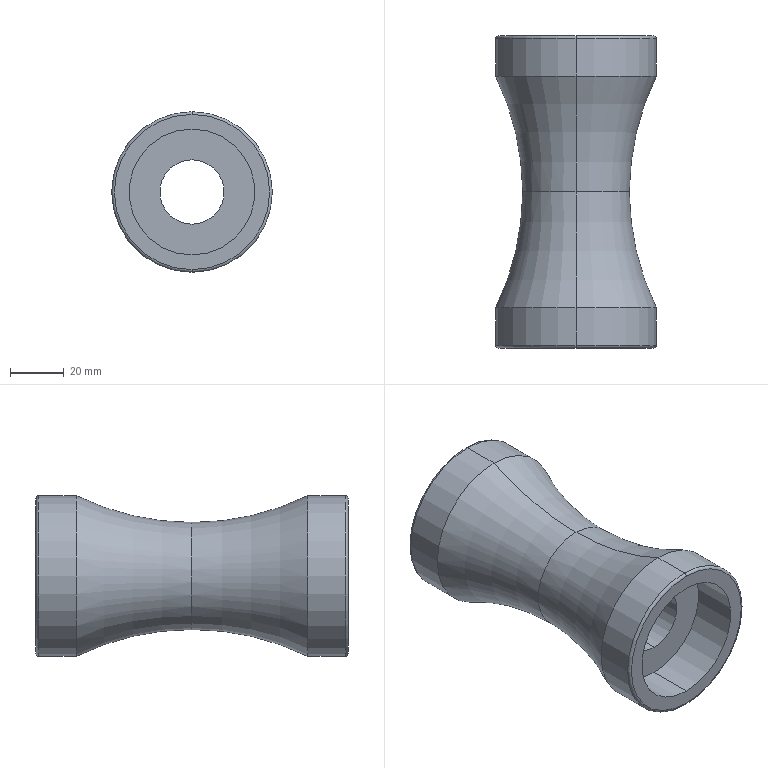Part | SolidWorks | features ICE 3, Fillet 1, Revolution 1 | 1 solid | 22 faces | box 60 x 116.5 x 60 mm | volume 137866 mm3 | cylinder 10 | torus 8 | plane 4 | commonest cylinder face diameters 47 x4 60 x4 24 x2
STEP:
#1=CARTESIAN_POINT('',(0.,15.,-30.));
#2=VERTEX_POINT('',#1);
#3=CARTESIAN_POINT('',(0.,58.25,-20.));
#4=VERTEX_POINT('',#3);
#5=CARTESIAN_POINT('',(0.,58.25,-118.528));
#6=DIRECTION('',(-1.,0.,0.));
#7=DIRECTION('',(0.,0.,1.));
#8=AXIS2_PLACEMENT_3D('',#5,#6,#7);
#9=CIRCLE('',#8,98.528);
#10=EDGE_CURVE('',#2,#4,#9,.T.);
#11=ORIENTED_EDGE('',*,*,#10,.T.);
#12=CARTESIAN_POINT('',(0.,58.25,20.));
#13=VERTEX_POINT('',#12);
#14=CARTESIAN_POINT('',(0.,58.25,0.));
#15=DIRECTION('',(0.,-1.,0.));
#16=DIRECTION('',(0.,0.,-1.));
#17=AXIS2_PLACEMENT_3D('',#14,#15,#16);
#18=CIRCLE('',#17,20.);
#19=EDGE_CURVE('',#4,#13,#18,.T.);
#20=ORIENTED_EDGE('',*,*,#19,.T.);
#21=CARTESIAN_POINT('',(0.,15.,30.));
#22=VERTEX_POINT('',#21);
#23=CARTESIAN_POINT('',(0.,58.25,118.528));
#24=DIRECTION('',(1.,0.,0.));
#25=DIRECTION('',(0.,0.,-1.));
#26=AXIS2_PLACEMENT_3D('',#23,#24,#25);
#27=CIRCLE('',#26,98.528);
#28=EDGE_CURVE('',#22,#13,#27,.T.);
#29=ORIENTED_EDGE('',*,*,#28,.F.);
#30=CARTESIAN_POINT('',(0.,15.,0.));
#31=DIRECTION('',(0.,-1.,0.));
#32=DIRECTION('',(0.,0.,-1.));
#33=AXIS2_PLACEMENT_3D('',#30,#31,#32);
#34=CIRCLE('',#33,30.);
#35=EDGE_CURVE('',#2,#22,#34,.T.);
#36=ORIENTED_EDGE('',*,*,#35,.F.);
#37=EDGE_LOOP('',(#11,#20,#29,#36));
#38=FACE_OUTER_BOUND('',#37,.T.);
#39=CARTESIAN_POINT('',(0.,58.25,0.));
#40=DIRECTION('',(0.,-1.,0.));
#41=DIRECTION('',(0.,0.,-1.));
#42=AXIS2_PLACEMENT_3D('',#39,#40,#41);
#43=TOROIDAL_SURFACE('',#42,118.528,98.528);
#44=ADVANCED_FACE('',(#38),#43,.F.);
#45=ORIENTED_EDGE('',*,*,#28,.T.);
#46=CARTESIAN_POINT('',(0.,58.25,0.));
#47=DIRECTION('',(0.,-1.,0.));
#48=DIRECTION('',(0.,0.,-1.));
#49=AXIS2_PLACEMENT_3D('',#46,#47,#48);
#50=CIRCLE('',#49,20.);
#51=EDGE_CURVE('',#13,#4,#50,.T.);
#52=ORIENTED_EDGE('',*,*,#51,.T.);
#53=ORIENTED_EDGE('',*,*,#10,.F.);
#54=CARTESIAN_POINT('',(0.,15.,0.));
#55=DIRECTION('',(0.,-1.,0.));
#56=DIRECTION('',(0.,0.,-1.));
#57=AXIS2_PLACEMENT_3D('',#54,#55,#56);
#58=CIRCLE('',#57,30.);
#59=EDGE_CURVE('',#22,#2,#58,.T.);
#60=ORIENTED_EDGE('',*,*,#59,.F.);
#61=EDGE_LOOP('',(#45,#52,#53,#60));
#62=FACE_OUTER_BOUND('',#61,.T.);
#63=CARTESIAN_POINT('',(0.,58.25,0.));
#64=DIRECTION('',(0.,-1.,0.));
#65=DIRECTION('',(0.,0.,-1.));
#66=AXIS2_PLACEMENT_3D('',#63,#64,#65);
#67=TOROIDAL_SURFACE('',#66,118.528,98.528);
#68=ADVANCED_FACE('',(#62),#67,.F.);
#69=CARTESIAN_POINT('',(0.,1.,30.));
#70=VERTEX_POINT('',#69);
#71=CARTESIAN_POINT('',(0.,1.,-30.));
#72=VERTEX_POINT('',#71);
#73=CARTESIAN_POINT('',(0.,1.,0.));
#74=DIRECTION('',(0.,1.,0.));
#75=DIRECTION('',(0.,0.,-1.));
#76=AXIS2_PLACEMENT_3D('',#73,#74,#75);
#77=CIRCLE('',#76,30.);
#78=EDGE_CURVE('',#70,#72,#77,.T.);
#79=ORIENTED_EDGE('',*,*,#78,.F.);
#80=CARTESIAN_POINT('',(0.,0.,29.));
#81=VERTEX_POINT('',#80);
#82=CARTESIAN_POINT('',(0.,1.,29.));
#83=DIRECTION('',(1.,0.,0.));
#84=DIRECTION('',(0.,0.,-1.));
#85=AXIS2_PLACEMENT_3D('',#82,#83,#84);
#86=CIRCLE('',#85,1.);
#87=EDGE_CURVE('',#70,#81,#86,.T.);
#88=ORIENTED_EDGE('',*,*,#87,.T.);
#89=CARTESIAN_POINT('',(0.,0.,-29.));
#90=VERTEX_POINT('',#89);
#91=CARTESIAN_POINT('',(0.,0.,0.));
#92=DIRECTION('',(0.,-1.,0.));
#93=DIRECTION('',(0.,0.,-1.));
#94=AXIS2_PLACEMENT_3D('',#91,#92,#93);
#95=CIRCLE('',#94,29.);
#96=EDGE_CURVE('',#90,#81,#95,.T.);
#97=ORIENTED_EDGE('',*,*,#96,.F.);
#98=CARTESIAN_POINT('',(0.,1.,-29.));
#99=DIRECTION('',(-1.,0.,0.));
#100=DIRECTION('',(0.,0.,1.));
#101=AXIS2_PLACEMENT_3D('',#98,#99,#100);
#102=CIRCLE('',#101,1.);
#103=EDGE_CURVE('',#72,#90,#102,.T.);
#104=ORIENTED_EDGE('',*,*,#103,.F.);
#105=EDGE_LOOP('',(#79,#88,#97,#104));
#106=FACE_OUTER_BOUND('',#105,.T.);
#107=CARTESIAN_POINT('',(0.,1.,0.));
#108=DIRECTION('',(0.,-1.,0.));
#109=DIRECTION('',(0.,0.,-1.));
#110=AXIS2_PLACEMENT_3D('',#107,#108,#109);
#111=TOROIDAL_SURFACE('',#110,29.,1.);
#112=ADVANCED_FACE('',(#106),#111,.T.);
#113=CARTESIAN_POINT('',(0.,115.5,-30.));
#114=VERTEX_POINT('',#113);
#115=CARTESIAN_POINT('',(0.,115.5,30.));
#116=VERTEX_POINT('',#115);
#117=CARTESIAN_POINT('',(0.,115.5,0.));
#118=DIRECTION('',(0.,-1.,0.));
#119=DIRECTION('',(0.,0.,1.));
#120=AXIS2_PLACEMENT_3D('',#117,#118,#119);
#121=CIRCLE('',#120,30.);
#122=EDGE_CURVE('',#114,#116,#121,.T.);
#123=ORIENTED_EDGE('',*,*,#122,.F.);
#124=CARTESIAN_POINT('',(0.,116.5,-29.));
#125=VERTEX_POINT('',#124);
#126=CARTESIAN_POINT('',(0.,115.5,-29.));
#127=DIRECTION('',(1.,0.,0.));
#128=DIRECTION('',(0.,0.,-1.));
#129=AXIS2_PLACEMENT_3D('',#126,#127,#128);
#130=CIRCLE('',#129,1.);
#131=EDGE_CURVE('',#114,#125,#130,.T.);
#132=ORIENTED_EDGE('',*,*,#131,.T.);
#133=CARTESIAN_POINT('',(0.,116.5,29.));
#134=VERTEX_POINT('',#133);
#135=CARTESIAN_POINT('',(0.,116.5,0.));
#136=DIRECTION('',(0.,1.,0.));
#137=DIRECTION('',(0.,0.,1.));
#138=AXIS2_PLACEMENT_3D('',#135,#136,#137);
#139=CIRCLE('',#138,29.);
#140=EDGE_CURVE('',#134,#125,#139,.T.);
#141=ORIENTED_EDGE('',*,*,#140,.F.);
#142=CARTESIAN_POINT('',(0.,115.5,29.));
#143=DIRECTION('',(-1.,0.,0.));
#144=DIRECTION('',(0.,0.,1.));
#145=AXIS2_PLACEMENT_3D('',#142,#143,#144);
#146=CIRCLE('',#145,1.);
#147=EDGE_CURVE('',#116,#134,#146,.T.);
#148=ORIENTED_EDGE('',*,*,#147,.F.);
#149=EDGE_LOOP('',(#123,#132,#141,#148));
#150=FACE_OUTER_BOUND('',#149,.T.);
#151=CARTESIAN_POINT('',(0.,115.5,0.));
#152=DIRECTION('',(0.,1.,0.));
#153=DIRECTION('',(0.,0.,1.));
#154=AXIS2_PLACEMENT_3D('',#151,#152,#153);
#155=TOROIDAL_SURFACE('',#154,29.,1.);
#156=ADVANCED_FACE('',(#150),#155,.T.);
#157=CARTESIAN_POINT('',(0.,17.,23.5));
#158=VERTEX_POINT('',#157);
#159=CARTESIAN_POINT('',(0.,17.,-23.5));
#160=VERTEX_POINT('',#159);
#161=CARTESIAN_POINT('',(0.,17.,0.));
#162=DIRECTION('',(0.,-1.,0.));
#163=DIRECTION('',(0.,0.,-1.));
#164=AXIS2_PLACEMENT_3D('',#161,#162,#163);
#165=CIRCLE('',#164,23.5);
#166=EDGE_CURVE('',#158,#160,#165,.T.);
#167=ORIENTED_EDGE('',*,*,#166,.F.);
#168=CARTESIAN_POINT('',(0.,0.,23.5));
#169=VERTEX_POINT('',#168);
#170=CARTESIAN_POINT('',(0.,17.,23.5));
#171=DIRECTION('',(0.,-1.,0.));
#172=VECTOR('',#171,1000.);
#173=LINE('',#170,#172);
#174=EDGE_CURVE('',#158,#169,#173,.T.);
#175=ORIENTED_EDGE('',*,*,#174,.T.);
#176=CARTESIAN_POINT('',(0.,0.,-23.5));
#177=VERTEX_POINT('',#176);
#178=CARTESIAN_POINT('',(0.,0.,0.));
#179=DIRECTION('',(0.,-1.,0.));
#180=DIRECTION('',(0.,0.,-1.));
#181=AXIS2_PLACEMENT_3D('',#178,#179,#180);
#182=CIRCLE('',#181,23.5);
#183=EDGE_CURVE('',#169,#177,#182,.T.);
#184=ORIENTED_EDGE('',*,*,#183,.T.);
#185=CARTESIAN_POINT('',(0.,17.,-23.5));
#186=DIRECTION('',(0.,-1.,0.));
#187=VECTOR('',#186,1000.);
#188=LINE('',#185,#187);
#189=EDGE_CURVE('',#160,#177,#188,.T.);
#190=ORIENTED_EDGE('',*,*,#189,.F.);
#191=EDGE_LOOP('',(#167,#175,#184,#190));
#192=FACE_OUTER_BOUND('',#191,.T.);
#193=CARTESIAN_POINT('',(0.,17.,0.));
#194=DIRECTION('',(0.,-1.,0.));
#195=DIRECTION('',(0.,0.,-1.));
#196=AXIS2_PLACEMENT_3D('',#193,#194,#195);
#197=CYLINDRICAL_SURFACE('',#196,23.5);
#198=ADVANCED_FACE('',(#192),#197,.F.);
#199=CARTESIAN_POINT('',(0.,99.5,-23.5));
#200=VERTEX_POINT('',#199);
#201=CARTESIAN_POINT('',(0.,99.5,23.5));
#202=VERTEX_POINT('',#201);
#203=CARTESIAN_POINT('',(0.,99.5,0.));
#204=DIRECTION('',(0.,1.,0.));
#205=DIRECTION('',(0.,0.,1.));
#206=AXIS2_PLACEMENT_3D('',#203,#204,#205);
#207=CIRCLE('',#206,23.5);
#208=EDGE_CURVE('',#200,#202,#207,.T.);
#209=ORIENTED_EDGE('',*,*,#208,.F.);
#210=CARTESIAN_POINT('',(0.,116.5,-23.5));
#211=VERTEX_POINT('',#210);
#212=CARTESIAN_POINT('',(0.,99.5,-23.5));
#213=DIRECTION('',(0.,1.,0.));
#214=VECTOR('',#213,1000.);
#215=LINE('',#212,#214);
#216=EDGE_CURVE('',#200,#211,#215,.T.);
#217=ORIENTED_EDGE('',*,*,#216,.T.);
#218=CARTESIAN_POINT('',(0.,116.5,23.5));
#219=VERTEX_POINT('',#218);
#220=CARTESIAN_POINT('',(0.,116.5,0.));
#221=DIRECTION('',(0.,1.,0.));
#222=DIRECTION('',(0.,0.,1.));
#223=AXIS2_PLACEMENT_3D('',#220,#221,#222);
#224=CIRCLE('',#223,23.5);
#225=EDGE_CURVE('',#211,#219,#224,.T.);
#226=ORIENTED_EDGE('',*,*,#225,.T.);
#227=CARTESIAN_POINT('',(0.,99.5,23.5));
#228=DIRECTION('',(0.,1.,0.));
#229=VECTOR('',#228,1000.);
#230=LINE('',#227,#229);
#231=EDGE_CURVE('',#202,#219,#230,.T.);
#232=ORIENTED_EDGE('',*,*,#231,.F.);
#233=EDGE_LOOP('',(#209,#217,#226,#232));
#234=FACE_OUTER_BOUND('',#233,.T.);
#235=CARTESIAN_POINT('',(0.,99.5,0.));
#236=DIRECTION('',(0.,1.,0.));
#237=DIRECTION('',(0.,0.,1.));
#238=AXIS2_PLACEMENT_3D('',#235,#236,#237);
#239=CYLINDRICAL_SURFACE('',#238,23.5);
#240=ADVANCED_FACE('',(#234),#239,.F.);
#241=ORIENTED_EDGE('',*,*,#122,.T.);
#242=CARTESIAN_POINT('',(0.,101.5,30.));
#243=VERTEX_POINT('',#242);
#244=CARTESIAN_POINT('',(0.,0.,30.));
#245=DIRECTION('',(0.,-1.,0.));
#246=VECTOR('',#245,1000.);
#247=LINE('',#244,#246);
#248=EDGE_CURVE('',#116,#243,#247,.T.);
#249=ORIENTED_EDGE('',*,*,#248,.T.);
#250=CARTESIAN_POINT('',(0.,101.5,-30.));
#251=VERTEX_POINT('',#250);
#252=CARTESIAN_POINT('',(0.,101.5,0.));
#253=DIRECTION('',(0.,-1.,0.));
#254=DIRECTION('',(0.,0.,-1.));
#255=AXIS2_PLACEMENT_3D('',#252,#253,#254);
#256=CIRCLE('',#255,30.);
#257=EDGE_CURVE('',#251,#243,#256,.T.);
#258=ORIENTED_EDGE('',*,*,#257,.F.);
#259=CARTESIAN_POINT('',(0.,0.,-30.));
#260=DIRECTION('',(0.,-1.,0.));
#261=VECTOR('',#260,1000.);
#262=LINE('',#259,#261);
#263=EDGE_CURVE('',#114,#251,#262,.T.);
#264=ORIENTED_EDGE('',*,*,#263,.F.);
#265=EDGE_LOOP('',(#241,#249,#258,#264));
#266=FACE_OUTER_BOUND('',#265,.T.);
#267=CARTESIAN_POINT('',(0.,0.,0.));
#268=DIRECTION('',(0.,-1.,0.));
#269=DIRECTION('',(0.,0.,-1.));
#270=AXIS2_PLACEMENT_3D('',#267,#268,#269);
#271=CYLINDRICAL_SURFACE('',#270,30.);
#272=ADVANCED_FACE('',(#266),#271,.T.);
#273=ORIENTED_EDGE('',*,*,#51,.F.);
#274=CARTESIAN_POINT('',(0.,58.25,118.528));
#275=DIRECTION('',(1.,0.,0.));
#276=DIRECTION('',(0.,0.,-1.));
#277=AXIS2_PLACEMENT_3D('',#274,#275,#276);
#278=CIRCLE('',#277,98.528);
#279=EDGE_CURVE('',#13,#243,#278,.T.);
#280=ORIENTED_EDGE('',*,*,#279,.T.);
#281=CARTESIAN_POINT('',(0.,101.5,0.));
#282=DIRECTION('',(0.,-1.,0.));
#283=DIRECTION('',(0.,0.,-1.));
#284=AXIS2_PLACEMENT_3D('',#281,#282,#283);
#285=CIRCLE('',#284,30.);
#286=EDGE_CURVE('',#243,#251,#285,.T.);
#287=ORIENTED_EDGE('',*,*,#286,.T.);
#288=CARTESIAN_POINT('',(0.,58.25,-118.528));
#289=DIRECTION('',(-1.,0.,0.));
#290=DIRECTION('',(0.,0.,1.));
#291=AXIS2_PLACEMENT_3D('',#288,#289,#290);
#292=CIRCLE('',#291,98.528);
#293=EDGE_CURVE('',#4,#251,#292,.T.);
#294=ORIENTED_EDGE('',*,*,#293,.F.);
#295=EDGE_LOOP('',(#273,#280,#287,#294));
#296=FACE_OUTER_BOUND('',#295,.T.);
#297=CARTESIAN_POINT('',(0.,58.25,0.));
#298=DIRECTION('',(0.,-1.,0.));
#299=DIRECTION('',(0.,0.,-1.));
#300=AXIS2_PLACEMENT_3D('',#297,#298,#299);
#301=TOROIDAL_SURFACE('',#300,118.528,98.528);
#302=ADVANCED_FACE('',(#296),#301,.F.);
#303=ORIENTED_EDGE('',*,*,#35,.T.);
#304=CARTESIAN_POINT('',(0.,0.,30.));
#305=DIRECTION('',(0.,-1.,0.));
#306=VECTOR('',#305,1000.);
#307=LINE('',#304,#306);
#308=EDGE_CURVE('',#22,#70,#307,.T.);
#309=ORIENTED_EDGE('',*,*,#308,.T.);
#310=ORIENTED_EDGE('',*,*,#78,.T.);
#311=CARTESIAN_POINT('',(0.,0.,-30.));
#312=DIRECTION('',(0.,-1.,0.));
#313=VECTOR('',#312,1000.);
#314=LINE('',#311,#313);
#315=EDGE_CURVE('',#2,#72,#314,.T.);
#316=ORIENTED_EDGE('',*,*,#315,.F.);
#317=EDGE_LOOP('',(#303,#309,#310,#316));
#318=FACE_OUTER_BOUND('',#317,.T.);
#319=CARTESIAN_POINT('',(0.,0.,0.));
#320=DIRECTION('',(0.,-1.,0.));
#321=DIRECTION('',(0.,0.,-1.));
#322=AXIS2_PLACEMENT_3D('',#319,#320,#321);
#323=CYLINDRICAL_SURFACE('',#322,30.);
#324=ADVANCED_FACE('',(#318),#323,.T.);
#325=CARTESIAN_POINT('',(0.,17.,-12.));
#326=VERTEX_POINT('',#325);
#327=CARTESIAN_POINT('',(0.,17.,12.));
#328=VERTEX_POINT('',#327);
#329=CARTESIAN_POINT('',(0.,17.,0.));
#330=DIRECTION('',(0.,1.,0.));
#331=DIRECTION('',(0.,0.,-1.));
#332=AXIS2_PLACEMENT_3D('',#329,#330,#331);
#333=CIRCLE('',#332,12.);
#334=EDGE_CURVE('',#326,#328,#333,.T.);
#335=ORIENTED_EDGE('',*,*,#334,.F.);
#336=CARTESIAN_POINT('',(0.,99.5,-12.));
#337=VERTEX_POINT('',#336);
#338=CARTESIAN_POINT('',(0.,-33.941,-12.));
#339=DIRECTION('',(0.,1.,0.));
#340=VECTOR('',#339,1000.);
#341=LINE('',#338,#340);
#342=EDGE_CURVE('',#326,#337,#341,.T.);
#343=ORIENTED_EDGE('',*,*,#342,.T.);
#344=CARTESIAN_POINT('',(0.,99.5,12.));
#345=VERTEX_POINT('',#344);
#346=CARTESIAN_POINT('',(0.,99.5,0.));
#347=DIRECTION('',(0.,-1.,0.));
#348=DIRECTION('',(0.,0.,1.));
#349=AXIS2_PLACEMENT_3D('',#346,#347,#348);
#350=CIRCLE('',#349,12.);
#351=EDGE_CURVE('',#345,#337,#350,.T.);
#352=ORIENTED_EDGE('',*,*,#351,.F.);
#353=CARTESIAN_POINT('',(0.,-33.941,12.));
#354=DIRECTION('',(0.,1.,0.));
#355=VECTOR('',#354,1000.);
#356=LINE('',#353,#355);
#357=EDGE_CURVE('',#328,#345,#356,.T.);
#358=ORIENTED_EDGE('',*,*,#357,.F.);
#359=EDGE_LOOP('',(#335,#343,#352,#358));
#360=FACE_OUTER_BOUND('',#359,.T.);
#361=CARTESIAN_POINT('',(0.,-33.941,0.));
#362=DIRECTION('',(0.,1.,0.));
#363=DIRECTION('',(0.,0.,1.));
#364=AXIS2_PLACEMENT_3D('',#361,#362,#363);
#365=CYLINDRICAL_SURFACE('',#364,12.);
#366=ADVANCED_FACE('',(#360),#365,.F.);
#367=ORIENTED_EDGE('',*,*,#342,.F.);
#368=CARTESIAN_POINT('',(0.,17.,0.));
#369=DIRECTION('',(0.,1.,0.));
#370=DIRECTION('',(0.,0.,-1.));
#371=AXIS2_PLACEMENT_3D('',#368,#369,#370);
#372=CIRCLE('',#371,12.);
#373=EDGE_CURVE('',#328,#326,#372,.T.);
#374=ORIENTED_EDGE('',*,*,#373,.F.);
#375=ORIENTED_EDGE('',*,*,#357,.T.);
#376=CARTESIAN_POINT('',(0.,99.5,0.));
#377=DIRECTION('',(0.,-1.,0.));
#378=DIRECTION('',(0.,0.,1.));
#379=AXIS2_PLACEMENT_3D('',#376,#377,#378);
#380=CIRCLE('',#379,12.);
#381=EDGE_CURVE('',#337,#345,#380,.T.);
#382=ORIENTED_EDGE('',*,*,#381,.F.);
#383=EDGE_LOOP('',(#367,#374,#375,#382));
#384=FACE_OUTER_BOUND('',#383,.T.);
#385=CARTESIAN_POINT('',(0.,-33.941,0.));
#386=DIRECTION('',(0.,1.,0.));
#387=DIRECTION('',(0.,0.,1.));
#388=AXIS2_PLACEMENT_3D('',#385,#386,#387);
#389=CYLINDRICAL_SURFACE('',#388,12.);
#390=ADVANCED_FACE('',(#384),#389,.F.);
#391=ORIENTED_EDGE('',*,*,#96,.T.);
#392=CARTESIAN_POINT('',(0.,0.,0.));
#393=DIRECTION('',(0.,-1.,0.));
#394=DIRECTION('',(0.,0.,-1.));
#395=AXIS2_PLACEMENT_3D('',#392,#393,#394);
#396=CIRCLE('',#395,29.);
#397=EDGE_CURVE('',#81,#90,#396,.T.);
#398=ORIENTED_EDGE('',*,*,#397,.T.);
#399=EDGE_LOOP('',(#391,#398));
#400=FACE_OUTER_BOUND('',#399,.T.);
#401=CARTESIAN_POINT('',(0.,0.,0.));
#402=DIRECTION('',(0.,-1.,0.));
#403=DIRECTION('',(0.,0.,-1.));
#404=AXIS2_PLACEMENT_3D('',#401,#402,#403);
#405=CIRCLE('',#404,23.5);
#406=EDGE_CURVE('',#177,#169,#405,.T.);
#407=ORIENTED_EDGE('',*,*,#406,.F.);
#408=ORIENTED_EDGE('',*,*,#183,.F.);
#409=EDGE_LOOP('',(#407,#408));
#410=FACE_BOUND('',#409,.T.);
#411=CARTESIAN_POINT('',(0.,0.,0.));
#412=DIRECTION('',(0.,-1.,0.));
#413=DIRECTION('',(0.,0.,-1.));
#414=AXIS2_PLACEMENT_3D('',#411,#412,#413);
#415=PLANE('',#414);
#416=ADVANCED_FACE('',(#400,#410),#415,.T.);
#417=ORIENTED_EDGE('',*,*,#308,.F.);
#418=ORIENTED_EDGE('',*,*,#59,.T.);
#419=ORIENTED_EDGE('',*,*,#315,.T.);
#420=CARTESIAN_POINT('',(0.,1.,0.));
#421=DIRECTION('',(0.,1.,0.));
#422=DIRECTION('',(0.,0.,-1.));
#423=AXIS2_PLACEMENT_3D('',#420,#421,#422);
#424=CIRCLE('',#423,30.);
#425=EDGE_CURVE('',#72,#70,#424,.T.);
#426=ORIENTED_EDGE('',*,*,#425,.T.);
#427=EDGE_LOOP('',(#417,#418,#419,#426));
#428=FACE_OUTER_BOUND('',#427,.T.);
#429=CARTESIAN_POINT('',(0.,0.,0.));
#430=DIRECTION('',(0.,-1.,0.));
#431=DIRECTION('',(0.,0.,-1.));
#432=AXIS2_PLACEMENT_3D('',#429,#430,#431);
#433=CYLINDRICAL_SURFACE('',#432,30.);
#434=ADVANCED_FACE('',(#428),#433,.T.);
#435=ORIENTED_EDGE('',*,*,#19,.F.);
#436=ORIENTED_EDGE('',*,*,#293,.T.);
#437=ORIENTED_EDGE('',*,*,#257,.T.);
#438=ORIENTED_EDGE('',*,*,#279,.F.);
#439=EDGE_LOOP('',(#435,#436,#437,#438));
#440=FACE_OUTER_BOUND('',#439,.T.);
#441=CARTESIAN_POINT('',(0.,58.25,0.));
#442=DIRECTION('',(0.,-1.,0.));
#443=DIRECTION('',(0.,0.,-1.));
#444=AXIS2_PLACEMENT_3D('',#441,#442,#443);
#445=TOROIDAL_SURFACE('',#444,118.528,98.528);
#446=ADVANCED_FACE('',(#440),#445,.F.);
#447=ORIENTED_EDGE('',*,*,#248,.F.);
#448=CARTESIAN_POINT('',(0.,115.5,0.));
#449=DIRECTION('',(0.,-1.,0.));
#450=DIRECTION('',(0.,0.,1.));
#451=AXIS2_PLACEMENT_3D('',#448,#449,#450);
#452=CIRCLE('',#451,30.);
#453=EDGE_CURVE('',#116,#114,#452,.T.);
#454=ORIENTED_EDGE('',*,*,#453,.T.);
#455=ORIENTED_EDGE('',*,*,#263,.T.);
#456=ORIENTED_EDGE('',*,*,#286,.F.);
#457=EDGE_LOOP('',(#447,#454,#455,#456));
#458=FACE_OUTER_BOUND('',#457,.T.);
#459=CARTESIAN_POINT('',(0.,0.,0.));
#460=DIRECTION('',(0.,-1.,0.));
#461=DIRECTION('',(0.,0.,-1.));
#462=AXIS2_PLACEMENT_3D('',#459,#460,#461);
#463=CYLINDRICAL_SURFACE('',#462,30.);
#464=ADVANCED_FACE('',(#458),#463,.T.);
#465=ORIENTED_EDGE('',*,*,#140,.T.);
#466=CARTESIAN_POINT('',(0.,116.5,0.));
#467=DIRECTION('',(0.,1.,0.));
#468=DIRECTION('',(0.,0.,1.));
#469=AXIS2_PLACEMENT_3D('',#466,#467,#468);
#470=CIRCLE('',#469,29.);
#471=EDGE_CURVE('',#125,#134,#470,.T.);
#472=ORIENTED_EDGE('',*,*,#471,.T.);
#473=EDGE_LOOP('',(#465,#472));
#474=FACE_OUTER_BOUND('',#473,.T.);
#475=CARTESIAN_POINT('',(0.,116.5,0.));
#476=DIRECTION('',(0.,1.,0.));
#477=DIRECTION('',(0.,0.,1.));
#478=AXIS2_PLACEMENT_3D('',#475,#476,#477);
#479=CIRCLE('',#478,23.5);
#480=EDGE_CURVE('',#219,#211,#479,.T.);
#481=ORIENTED_EDGE('',*,*,#480,.F.);
#482=ORIENTED_EDGE('',*,*,#225,.F.);
#483=EDGE_LOOP('',(#481,#482));
#484=FACE_BOUND('',#483,.T.);
#485=CARTESIAN_POINT('',(0.,116.5,0.));
#486=DIRECTION('',(0.,1.,0.));
#487=DIRECTION('',(0.,0.,1.));
#488=AXIS2_PLACEMENT_3D('',#485,#486,#487);
#489=PLANE('',#488);
#490=ADVANCED_FACE('',(#474,#484),#489,.T.);
#491=CARTESIAN_POINT('',(0.,99.5,0.));
#492=DIRECTION('',(0.,1.,0.));
#493=DIRECTION('',(0.,0.,1.));
#494=AXIS2_PLACEMENT_3D('',#491,#492,#493);
#495=CIRCLE('',#494,23.5);
#496=EDGE_CURVE('',#202,#200,#495,.T.);
#497=ORIENTED_EDGE('',*,*,#496,.T.);
#498=ORIENTED_EDGE('',*,*,#208,.T.);
#499=EDGE_LOOP('',(#497,#498));
#500=FACE_OUTER_BOUND('',#499,.T.);
#501=ORIENTED_EDGE('',*,*,#351,.T.);
#502=ORIENTED_EDGE('',*,*,#381,.T.);
#503=EDGE_LOOP('',(#501,#502));
#504=FACE_BOUND('',#503,.T.);
#505=CARTESIAN_POINT('',(0.,99.5,0.));
#506=DIRECTION('',(0.,1.,0.));
#507=DIRECTION('',(0.,0.,1.));
#508=AXIS2_PLACEMENT_3D('',#505,#506,#507);
#509=PLANE('',#508);
#510=ADVANCED_FACE('',(#500,#504),#509,.T.);
#511=ORIENTED_EDGE('',*,*,#216,.F.);
#512=ORIENTED_EDGE('',*,*,#496,.F.);
#513=ORIENTED_EDGE('',*,*,#231,.T.);
#514=ORIENTED_EDGE('',*,*,#480,.T.);
#515=EDGE_LOOP('',(#511,#512,#513,#514));
#516=FACE_OUTER_BOUND('',#515,.T.);
#517=CARTESIAN_POINT('',(0.,99.5,0.));
#518=DIRECTION('',(0.,1.,0.));
#519=DIRECTION('',(0.,0.,1.));
#520=AXIS2_PLACEMENT_3D('',#517,#518,#519);
#521=CYLINDRICAL_SURFACE('',#520,23.5);
#522=ADVANCED_FACE('',(#516),#521,.F.);
#523=CARTESIAN_POINT('',(0.,17.,0.));
#524=DIRECTION('',(0.,-1.,0.));
#525=DIRECTION('',(0.,0.,-1.));
#526=AXIS2_PLACEMENT_3D('',#523,#524,#525);
#527=CIRCLE('',#526,23.5);
#528=EDGE_CURVE('',#160,#158,#527,.T.);
#529=ORIENTED_EDGE('',*,*,#528,.T.);
#530=ORIENTED_EDGE('',*,*,#166,.T.);
#531=EDGE_LOOP('',(#529,#530));
#532=FACE_OUTER_BOUND('',#531,.T.);
#533=ORIENTED_EDGE('',*,*,#373,.T.);
#534=ORIENTED_EDGE('',*,*,#334,.T.);
#535=EDGE_LOOP('',(#533,#534));
#536=FACE_BOUND('',#535,.T.);
#537=CARTESIAN_POINT('',(0.,17.,0.));
#538=DIRECTION('',(0.,-1.,0.));
#539=DIRECTION('',(0.,0.,-1.));
#540=AXIS2_PLACEMENT_3D('',#537,#538,#539);
#541=PLANE('',#540);
#542=ADVANCED_FACE('',(#532,#536),#541,.T.);
#543=ORIENTED_EDGE('',*,*,#174,.F.);
#544=ORIENTED_EDGE('',*,*,#528,.F.);
#545=ORIENTED_EDGE('',*,*,#189,.T.);
#546=ORIENTED_EDGE('',*,*,#406,.T.);
#547=EDGE_LOOP('',(#543,#544,#545,#546));
#548=FACE_OUTER_BOUND('',#547,.T.);
#549=CARTESIAN_POINT('',(0.,17.,0.));
#550=DIRECTION('',(0.,-1.,0.));
#551=DIRECTION('',(0.,0.,-1.));
#552=AXIS2_PLACEMENT_3D('',#549,#550,#551);
#553=CYLINDRICAL_SURFACE('',#552,23.5);
#554=ADVANCED_FACE('',(#548),#553,.F.);
#555=ORIENTED_EDGE('',*,*,#131,.F.);
#556=ORIENTED_EDGE('',*,*,#453,.F.);
#557=ORIENTED_EDGE('',*,*,#147,.T.);
#558=ORIENTED_EDGE('',*,*,#471,.F.);
#559=EDGE_LOOP('',(#555,#556,#557,#558));
#560=FACE_OUTER_BOUND('',#559,.T.);
#561=CARTESIAN_POINT('',(0.,115.5,0.));
#562=DIRECTION('',(0.,1.,0.));
#563=DIRECTION('',(0.,0.,1.));
#564=AXIS2_PLACEMENT_3D('',#561,#562,#563);
#565=TOROIDAL_SURFACE('',#564,29.,1.);
#566=ADVANCED_FACE('',(#560),#565,.T.);
#567=ORIENTED_EDGE('',*,*,#87,.F.);
#568=ORIENTED_EDGE('',*,*,#425,.F.);
#569=ORIENTED_EDGE('',*,*,#103,.T.);
#570=ORIENTED_EDGE('',*,*,#397,.F.);
#571=EDGE_LOOP('',(#567,#568,#569,#570));
#572=FACE_OUTER_BOUND('',#571,.T.);
#573=CARTESIAN_POINT('',(0.,1.,0.));
#574=DIRECTION('',(0.,-1.,0.));
#575=DIRECTION('',(0.,0.,-1.));
#576=AXIS2_PLACEMENT_3D('',#573,#574,#575);
#577=TOROIDAL_SURFACE('',#576,29.,1.);
#578=ADVANCED_FACE('',(#572),#577,.T.);
#579=CLOSED_SHELL('',(#44,#68,#112,#156,#198,#240,#272,#302,#324,#366,#390,#416,#434,#446,#464,#490,#510,#522,#542,#554,#566,#578));
#580=MANIFOLD_SOLID_BREP('',#579);
#581=CARTESIAN_POINT('',(0.,0.,0.));
#582=DIRECTION('',(0.,0.,1.));
#583=DIRECTION('',(1.,0.,0.));
#584=AXIS2_PLACEMENT_3D('',#581,#582,#583);
#585=(LENGTH_UNIT()NAMED_UNIT(*)SI_UNIT(.MILLI.,.METRE.));
#586=UNCERTAINTY_MEASURE_WITH_UNIT(LENGTH_MEASURE(0.00001),#585,'','');
#587=(NAMED_UNIT(*)PLANE_ANGLE_UNIT()SI_UNIT($,.RADIAN.));
#588=(NAMED_UNIT(*)SI_UNIT($,.STERADIAN.)SOLID_ANGLE_UNIT());
#589=(GEOMETRIC_REPRESENTATION_CONTEXT(3)GLOBAL_UNCERTAINTY_ASSIGNED_CONTEXT((#586))GLOBAL_UNIT_ASSIGNED_CONTEXT((#585,#587,#588))REPRESENTATION_CONTEXT('',''));
#590=ADVANCED_BREP_SHAPE_REPRESENTATION('',(#580,#584),#589);